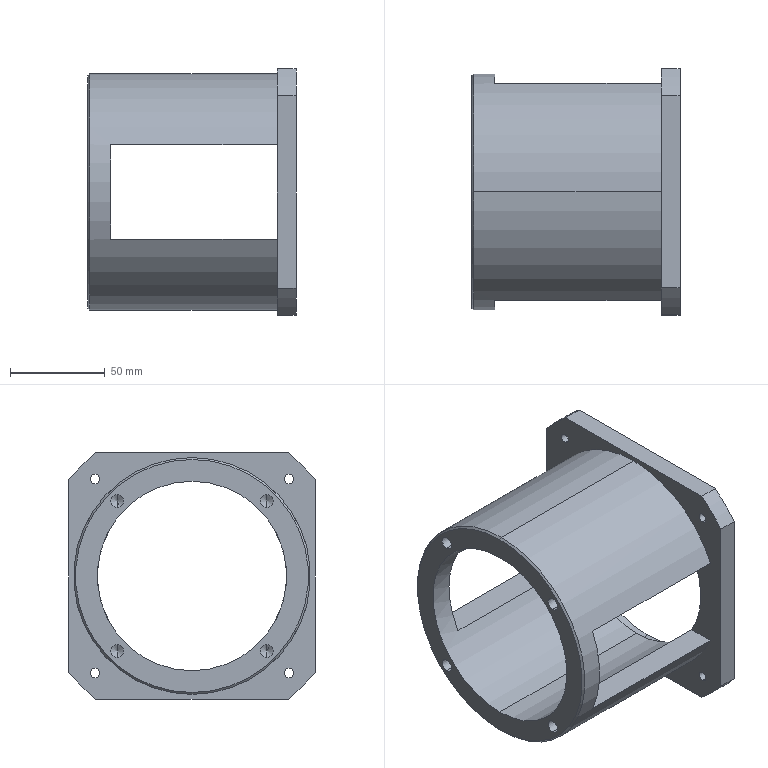Part | SolidWorks | features ICE 5, CirPattern 2, HoleWzd 2, Chamfer 1, Extrusion 1 | 1 solid | 50 faces | box 110 x 130 x 130 mm | volume 397352 mm3 | cylinder 26 | plane 14 | cone 10 | commonest cylinder face diameters 5 x8 6.8 x8 165 x4 100 x2 110 x2 125 x2
STEP:
#1=CARTESIAN_POINT('',(0.,0.,61.5));
#2=VERTEX_POINT('',#1);
#3=CARTESIAN_POINT('',(0.,0.,-61.5));
#4=VERTEX_POINT('',#3);
#5=CARTESIAN_POINT('',(0.,0.,0.));
#6=DIRECTION('',(-1.,0.,0.));
#7=DIRECTION('',(0.,0.,-1.));
#8=AXIS2_PLACEMENT_3D('',#5,#6,#7);
#9=CIRCLE('',#8,61.5);
#10=EDGE_CURVE('',#2,#4,#9,.T.);
#11=ORIENTED_EDGE('',*,*,#10,.F.);
#12=CARTESIAN_POINT('',(1.,0.,62.5));
#13=VERTEX_POINT('',#12);
#14=CARTESIAN_POINT('',(1.,0.,62.5));
#15=DIRECTION('',(0.7071,0.,0.7071));
#16=VECTOR('',#15,1000.);
#17=LINE('',#14,#16);
#18=EDGE_CURVE('',#2,#13,#17,.T.);
#19=ORIENTED_EDGE('',*,*,#18,.T.);
#20=CARTESIAN_POINT('',(1.,0.,-62.5));
#21=VERTEX_POINT('',#20);
#22=CARTESIAN_POINT('',(1.,0.,0.));
#23=DIRECTION('',(1.,0.,0.));
#24=DIRECTION('',(0.,0.,-1.));
#25=AXIS2_PLACEMENT_3D('',#22,#23,#24);
#26=CIRCLE('',#25,62.5);
#27=EDGE_CURVE('',#21,#13,#26,.T.);
#28=ORIENTED_EDGE('',*,*,#27,.F.);
#29=CARTESIAN_POINT('',(1.,0.,-62.5));
#30=DIRECTION('',(0.7071,0.,-0.7071));
#31=VECTOR('',#30,1000.);
#32=LINE('',#29,#31);
#33=EDGE_CURVE('',#4,#21,#32,.T.);
#34=ORIENTED_EDGE('',*,*,#33,.F.);
#35=EDGE_LOOP('',(#11,#19,#28,#34));
#36=FACE_OUTER_BOUND('',#35,.T.);
#37=CARTESIAN_POINT('',(1.,0.,0.));
#38=DIRECTION('',(1.,0.,0.));
#39=DIRECTION('',(0.,0.,-1.));
#40=AXIS2_PLACEMENT_3D('',#37,#38,#39);
#41=CONICAL_SURFACE('',#40,62.5,0.7854);
#42=ADVANCED_FACE('',(#36),#41,.T.);
#43=CARTESIAN_POINT('',(19.75,-39.598,-42.998));
#44=VERTEX_POINT('',#43);
#45=CARTESIAN_POINT('',(19.75,-39.598,-36.198));
#46=VERTEX_POINT('',#45);
#47=CARTESIAN_POINT('',(19.75,-39.598,-39.598));
#48=DIRECTION('',(-1.,0.,0.));
#49=DIRECTION('',(0.,0.,1.));
#50=AXIS2_PLACEMENT_3D('',#47,#48,#49);
#51=CIRCLE('',#50,3.4);
#52=EDGE_CURVE('',#44,#46,#51,.T.);
#53=ORIENTED_EDGE('',*,*,#52,.F.);
#54=CARTESIAN_POINT('',(0.,-39.598,-42.998));
#55=VERTEX_POINT('',#54);
#56=CARTESIAN_POINT('',(0.,-39.598,-42.998));
#57=DIRECTION('',(-1.,0.,0.));
#58=VECTOR('',#57,1000.);
#59=LINE('',#56,#58);
#60=EDGE_CURVE('',#44,#55,#59,.T.);
#61=ORIENTED_EDGE('',*,*,#60,.T.);
#62=CARTESIAN_POINT('',(0.,-39.598,-36.198));
#63=VERTEX_POINT('',#62);
#64=CARTESIAN_POINT('',(0.,-39.598,-39.598));
#65=DIRECTION('',(-1.,0.,0.));
#66=DIRECTION('',(0.,0.,1.));
#67=AXIS2_PLACEMENT_3D('',#64,#65,#66);
#68=CIRCLE('',#67,3.4);
#69=EDGE_CURVE('',#55,#63,#68,.T.);
#70=ORIENTED_EDGE('',*,*,#69,.T.);
#71=CARTESIAN_POINT('',(0.,-39.598,-36.198));
#72=DIRECTION('',(-1.,0.,0.));
#73=VECTOR('',#72,1000.);
#74=LINE('',#71,#73);
#75=EDGE_CURVE('',#46,#63,#74,.T.);
#76=ORIENTED_EDGE('',*,*,#75,.F.);
#77=EDGE_LOOP('',(#53,#61,#70,#76));
#78=FACE_OUTER_BOUND('',#77,.T.);
#79=CARTESIAN_POINT('',(0.,-39.598,-39.598));
#80=DIRECTION('',(-1.,0.,0.));
#81=DIRECTION('',(0.,0.,1.));
#82=AXIS2_PLACEMENT_3D('',#79,#80,#81);
#83=CYLINDRICAL_SURFACE('',#82,3.4);
#84=ADVANCED_FACE('',(#78),#83,.F.);
#85=CARTESIAN_POINT('',(21.793,-39.598,-39.598));
#86=VERTEX_POINT('',#85);
#87=CARTESIAN_POINT('',(19.75,-39.598,-36.198));
#88=DIRECTION('',(-0.515,0.,0.8572));
#89=VECTOR('',#88,1000.);
#90=LINE('',#87,#89);
#91=EDGE_CURVE('',#86,#46,#90,.T.);
#92=ORIENTED_EDGE('',*,*,#91,.F.);
#93=CARTESIAN_POINT('',(19.75,-39.598,-42.998));
#94=DIRECTION('',(-0.515,0.,-0.8572));
#95=VECTOR('',#94,1000.);
#96=LINE('',#93,#95);
#97=EDGE_CURVE('',#86,#44,#96,.T.);
#98=ORIENTED_EDGE('',*,*,#97,.T.);
#99=ORIENTED_EDGE('',*,*,#52,.T.);
#100=EDGE_LOOP('',(#92,#98,#99));
#101=FACE_OUTER_BOUND('',#100,.T.);
#102=CARTESIAN_POINT('',(19.75,-39.598,-39.598));
#103=DIRECTION('',(-1.,0.,0.));
#104=DIRECTION('',(0.,0.,1.));
#105=AXIS2_PLACEMENT_3D('',#102,#103,#104);
#106=CONICAL_SURFACE('',#105,3.4,1.03);
#107=ADVANCED_FACE('',(#101),#106,.F.);
#108=CARTESIAN_POINT('',(19.75,-39.598,36.198));
#109=VERTEX_POINT('',#108);
#110=CARTESIAN_POINT('',(19.75,-39.598,42.998));
#111=VERTEX_POINT('',#110);
#112=CARTESIAN_POINT('',(19.75,-39.598,39.598));
#113=DIRECTION('',(-1.,0.,0.));
#114=DIRECTION('',(0.,0.,1.));
#115=AXIS2_PLACEMENT_3D('',#112,#113,#114);
#116=CIRCLE('',#115,3.4);
#117=EDGE_CURVE('',#109,#111,#116,.T.);
#118=ORIENTED_EDGE('',*,*,#117,.F.);
#119=CARTESIAN_POINT('',(0.,-39.598,36.198));
#120=VERTEX_POINT('',#119);
#121=CARTESIAN_POINT('',(0.,-39.598,36.198));
#122=DIRECTION('',(-1.,0.,0.));
#123=VECTOR('',#122,1000.);
#124=LINE('',#121,#123);
#125=EDGE_CURVE('',#109,#120,#124,.T.);
#126=ORIENTED_EDGE('',*,*,#125,.T.);
#127=CARTESIAN_POINT('',(0.,-39.598,42.998));
#128=VERTEX_POINT('',#127);
#129=CARTESIAN_POINT('',(0.,-39.598,39.598));
#130=DIRECTION('',(-1.,0.,0.));
#131=DIRECTION('',(0.,0.,1.));
#132=AXIS2_PLACEMENT_3D('',#129,#130,#131);
#133=CIRCLE('',#132,3.4);
#134=EDGE_CURVE('',#120,#128,#133,.T.);
#135=ORIENTED_EDGE('',*,*,#134,.T.);
#136=CARTESIAN_POINT('',(0.,-39.598,42.998));
#137=DIRECTION('',(-1.,0.,0.));
#138=VECTOR('',#137,1000.);
#139=LINE('',#136,#138);
#140=EDGE_CURVE('',#111,#128,#139,.T.);
#141=ORIENTED_EDGE('',*,*,#140,.F.);
#142=EDGE_LOOP('',(#118,#126,#135,#141));
#143=FACE_OUTER_BOUND('',#142,.T.);
#144=CARTESIAN_POINT('',(0.,-39.598,39.598));
#145=DIRECTION('',(-1.,0.,0.));
#146=DIRECTION('',(0.,0.,1.));
#147=AXIS2_PLACEMENT_3D('',#144,#145,#146);
#148=CYLINDRICAL_SURFACE('',#147,3.4);
#149=ADVANCED_FACE('',(#143),#148,.F.);
#150=CARTESIAN_POINT('',(21.793,-39.598,39.598));
#151=VERTEX_POINT('',#150);
#152=CARTESIAN_POINT('',(19.75,-39.598,42.998));
#153=DIRECTION('',(-0.515,0.,0.8572));
#154=VECTOR('',#153,1000.);
#155=LINE('',#152,#154);
#156=EDGE_CURVE('',#151,#111,#155,.T.);
#157=ORIENTED_EDGE('',*,*,#156,.F.);
#158=CARTESIAN_POINT('',(19.75,-39.598,36.198));
#159=DIRECTION('',(-0.515,0.,-0.8572));
#160=VECTOR('',#159,1000.);
#161=LINE('',#158,#160);
#162=EDGE_CURVE('',#151,#109,#161,.T.);
#163=ORIENTED_EDGE('',*,*,#162,.T.);
#164=ORIENTED_EDGE('',*,*,#117,.T.);
#165=EDGE_LOOP('',(#157,#163,#164));
#166=FACE_OUTER_BOUND('',#165,.T.);
#167=CARTESIAN_POINT('',(19.75,-39.598,39.598));
#168=DIRECTION('',(-1.,0.,0.));
#169=DIRECTION('',(0.,0.,1.));
#170=AXIS2_PLACEMENT_3D('',#167,#168,#169);
#171=CONICAL_SURFACE('',#170,3.4,1.03);
#172=ADVANCED_FACE('',(#166),#171,.F.);
#173=CARTESIAN_POINT('',(19.75,39.598,36.198));
#174=VERTEX_POINT('',#173);
#175=CARTESIAN_POINT('',(19.75,39.598,42.998));
#176=VERTEX_POINT('',#175);
#177=CARTESIAN_POINT('',(19.75,39.598,39.598));
#178=DIRECTION('',(-1.,0.,0.));
#179=DIRECTION('',(0.,0.,1.));
#180=AXIS2_PLACEMENT_3D('',#177,#178,#179);
#181=CIRCLE('',#180,3.4);
#182=EDGE_CURVE('',#174,#176,#181,.T.);
#183=ORIENTED_EDGE('',*,*,#182,.F.);
#184=CARTESIAN_POINT('',(0.,39.598,36.198));
#185=VERTEX_POINT('',#184);
#186=CARTESIAN_POINT('',(0.,39.598,36.198));
#187=DIRECTION('',(-1.,0.,0.));
#188=VECTOR('',#187,1000.);
#189=LINE('',#186,#188);
#190=EDGE_CURVE('',#174,#185,#189,.T.);
#191=ORIENTED_EDGE('',*,*,#190,.T.);
#192=CARTESIAN_POINT('',(0.,39.598,42.998));
#193=VERTEX_POINT('',#192);
#194=CARTESIAN_POINT('',(0.,39.598,39.598));
#195=DIRECTION('',(-1.,0.,0.));
#196=DIRECTION('',(0.,0.,1.));
#197=AXIS2_PLACEMENT_3D('',#194,#195,#196);
#198=CIRCLE('',#197,3.4);
#199=EDGE_CURVE('',#185,#193,#198,.T.);
#200=ORIENTED_EDGE('',*,*,#199,.T.);
#201=CARTESIAN_POINT('',(0.,39.598,42.998));
#202=DIRECTION('',(-1.,0.,0.));
#203=VECTOR('',#202,1000.);
#204=LINE('',#201,#203);
#205=EDGE_CURVE('',#176,#193,#204,.T.);
#206=ORIENTED_EDGE('',*,*,#205,.F.);
#207=EDGE_LOOP('',(#183,#191,#200,#206));
#208=FACE_OUTER_BOUND('',#207,.T.);
#209=CARTESIAN_POINT('',(0.,39.598,39.598));
#210=DIRECTION('',(-1.,0.,0.));
#211=DIRECTION('',(0.,0.,1.));
#212=AXIS2_PLACEMENT_3D('',#209,#210,#211);
#213=CYLINDRICAL_SURFACE('',#212,3.4);
#214=ADVANCED_FACE('',(#208),#213,.F.);
#215=CARTESIAN_POINT('',(21.793,39.598,39.598));
#216=VERTEX_POINT('',#215);
#217=CARTESIAN_POINT('',(19.75,39.598,42.998));
#218=DIRECTION('',(-0.515,0.,0.8572));
#219=VECTOR('',#218,1000.);
#220=LINE('',#217,#219);
#221=EDGE_CURVE('',#216,#176,#220,.T.);
#222=ORIENTED_EDGE('',*,*,#221,.F.);
#223=CARTESIAN_POINT('',(19.75,39.598,36.198));
#224=DIRECTION('',(-0.515,0.,-0.8572));
#225=VECTOR('',#224,1000.);
#226=LINE('',#223,#225);
#227=EDGE_CURVE('',#216,#174,#226,.T.);
#228=ORIENTED_EDGE('',*,*,#227,.T.);
#229=ORIENTED_EDGE('',*,*,#182,.T.);
#230=EDGE_LOOP('',(#222,#228,#229));
#231=FACE_OUTER_BOUND('',#230,.T.);
#232=CARTESIAN_POINT('',(19.75,39.598,39.598));
#233=DIRECTION('',(-1.,0.,0.));
#234=DIRECTION('',(0.,0.,1.));
#235=AXIS2_PLACEMENT_3D('',#232,#233,#234);
#236=CONICAL_SURFACE('',#235,3.4,1.03);
#237=ADVANCED_FACE('',(#231),#236,.F.);
#238=CARTESIAN_POINT('',(19.75,39.598,-42.998));
#239=VERTEX_POINT('',#238);
#240=CARTESIAN_POINT('',(19.75,39.598,-36.198));
#241=VERTEX_POINT('',#240);
#242=CARTESIAN_POINT('',(19.75,39.598,-39.598));
#243=DIRECTION('',(-1.,0.,0.));
#244=DIRECTION('',(0.,0.,1.));
#245=AXIS2_PLACEMENT_3D('',#242,#243,#244);
#246=CIRCLE('',#245,3.4);
#247=EDGE_CURVE('',#239,#241,#246,.T.);
#248=ORIENTED_EDGE('',*,*,#247,.F.);
#249=CARTESIAN_POINT('',(0.,39.598,-42.998));
#250=VERTEX_POINT('',#249);
#251=CARTESIAN_POINT('',(0.,39.598,-42.998));
#252=DIRECTION('',(-1.,0.,0.));
#253=VECTOR('',#252,1000.);
#254=LINE('',#251,#253);
#255=EDGE_CURVE('',#239,#250,#254,.T.);
#256=ORIENTED_EDGE('',*,*,#255,.T.);
#257=CARTESIAN_POINT('',(0.,39.598,-36.198));
#258=VERTEX_POINT('',#257);
#259=CARTESIAN_POINT('',(0.,39.598,-39.598));
#260=DIRECTION('',(-1.,0.,0.));
#261=DIRECTION('',(0.,0.,1.));
#262=AXIS2_PLACEMENT_3D('',#259,#260,#261);
#263=CIRCLE('',#262,3.4);
#264=EDGE_CURVE('',#250,#258,#263,.T.);
#265=ORIENTED_EDGE('',*,*,#264,.T.);
#266=CARTESIAN_POINT('',(0.,39.598,-36.198));
#267=DIRECTION('',(-1.,0.,0.));
#268=VECTOR('',#267,1000.);
#269=LINE('',#266,#268);
#270=EDGE_CURVE('',#241,#258,#269,.T.);
#271=ORIENTED_EDGE('',*,*,#270,.F.);
#272=EDGE_LOOP('',(#248,#256,#265,#271));
#273=FACE_OUTER_BOUND('',#272,.T.);
#274=CARTESIAN_POINT('',(0.,39.598,-39.598));
#275=DIRECTION('',(-1.,0.,0.));
#276=DIRECTION('',(0.,0.,1.));
#277=AXIS2_PLACEMENT_3D('',#274,#275,#276);
#278=CYLINDRICAL_SURFACE('',#277,3.4);
#279=ADVANCED_FACE('',(#273),#278,.F.);
#280=CARTESIAN_POINT('',(21.793,39.598,-39.598));
#281=VERTEX_POINT('',#280);
#282=CARTESIAN_POINT('',(19.75,39.598,-36.198));
#283=DIRECTION('',(-0.515,0.,0.8572));
#284=VECTOR('',#283,1000.);
#285=LINE('',#282,#284);
#286=EDGE_CURVE('',#281,#241,#285,.T.);
#287=ORIENTED_EDGE('',*,*,#286,.F.);
#288=CARTESIAN_POINT('',(19.75,39.598,-42.998));
#289=DIRECTION('',(-0.515,0.,-0.8572));
#290=VECTOR('',#289,1000.);
#291=LINE('',#288,#290);
#292=EDGE_CURVE('',#281,#239,#291,.T.);
#293=ORIENTED_EDGE('',*,*,#292,.T.);
#294=ORIENTED_EDGE('',*,*,#247,.T.);
#295=EDGE_LOOP('',(#287,#293,#294));
#296=FACE_OUTER_BOUND('',#295,.T.);
#297=CARTESIAN_POINT('',(19.75,39.598,-39.598));
#298=DIRECTION('',(-1.,0.,0.));
#299=DIRECTION('',(0.,0.,1.));
#300=AXIS2_PLACEMENT_3D('',#297,#298,#299);
#301=CONICAL_SURFACE('',#300,3.4,1.03);
#302=ADVANCED_FACE('',(#296),#301,.F.);
#303=CARTESIAN_POINT('',(100.,-43.301,25.));
#304=VERTEX_POINT('',#303);
#305=CARTESIAN_POINT('',(12.,-43.301,25.));
#306=VERTEX_POINT('',#305);
#307=CARTESIAN_POINT('',(0.,-43.301,25.));
#308=DIRECTION('',(-1.,0.,0.));
#309=VECTOR('',#308,1000.);
#310=LINE('',#307,#309);
#311=EDGE_CURVE('',#304,#306,#310,.T.);
#312=ORIENTED_EDGE('',*,*,#311,.T.);
#313=CARTESIAN_POINT('',(12.,-43.301,-25.));
#314=VERTEX_POINT('',#313);
#315=CARTESIAN_POINT('',(12.,0.,0.));
#316=DIRECTION('',(1.,0.,0.));
#317=DIRECTION('',(0.,0.,1.));
#318=AXIS2_PLACEMENT_3D('',#315,#316,#317);
#319=CIRCLE('',#318,50.);
#320=EDGE_CURVE('',#306,#314,#319,.T.);
#321=ORIENTED_EDGE('',*,*,#320,.T.);
#322=CARTESIAN_POINT('',(100.,-43.301,-25.));
#323=VERTEX_POINT('',#322);
#324=CARTESIAN_POINT('',(0.,-43.301,-25.));
#325=DIRECTION('',(1.,0.,0.));
#326=VECTOR('',#325,1000.);
#327=LINE('',#324,#326);
#328=EDGE_CURVE('',#314,#323,#327,.T.);
#329=ORIENTED_EDGE('',*,*,#328,.T.);
#330=CARTESIAN_POINT('',(100.,0.,0.));
#331=DIRECTION('',(-1.,0.,0.));
#332=DIRECTION('',(0.,0.,-1.));
#333=AXIS2_PLACEMENT_3D('',#330,#331,#332);
#334=CIRCLE('',#333,50.);
#335=EDGE_CURVE('',#323,#304,#334,.T.);
#336=ORIENTED_EDGE('',*,*,#335,.T.);
#337=EDGE_LOOP('',(#312,#321,#329,#336));
#338=FACE_BOUND('',#337,.T.);
#339=CARTESIAN_POINT('',(0.,0.,50.));
#340=VERTEX_POINT('',#339);
#341=CARTESIAN_POINT('',(0.,0.,-50.));
#342=VERTEX_POINT('',#341);
#343=CARTESIAN_POINT('',(0.,0.,0.));
#344=DIRECTION('',(1.,0.,0.));
#345=DIRECTION('',(0.,0.,-1.));
#346=AXIS2_PLACEMENT_3D('',#343,#344,#345);
#347=CIRCLE('',#346,50.);
#348=EDGE_CURVE('',#340,#342,#347,.T.);
#349=ORIENTED_EDGE('',*,*,#348,.F.);
#350=CARTESIAN_POINT('',(102.,0.,50.));
#351=VERTEX_POINT('',#350);
#352=CARTESIAN_POINT('',(0.,0.,50.));
#353=DIRECTION('',(1.,0.,0.));
#354=VECTOR('',#353,1000.);
#355=LINE('',#352,#354);
#356=EDGE_CURVE('',#340,#351,#355,.T.);
#357=ORIENTED_EDGE('',*,*,#356,.T.);
#358=CARTESIAN_POINT('',(102.,0.,-50.));
#359=VERTEX_POINT('',#358);
#360=CARTESIAN_POINT('',(102.,0.,0.));
#361=DIRECTION('',(1.,0.,0.));
#362=DIRECTION('',(0.,0.,-1.));
#363=AXIS2_PLACEMENT_3D('',#360,#361,#362);
#364=CIRCLE('',#363,50.);
#365=EDGE_CURVE('',#351,#359,#364,.T.);
#366=ORIENTED_EDGE('',*,*,#365,.T.);
#367=CARTESIAN_POINT('',(0.,0.,-50.));
#368=DIRECTION('',(1.,0.,0.));
#369=VECTOR('',#368,1000.);
#370=LINE('',#367,#369);
#371=EDGE_CURVE('',#342,#359,#370,.T.);
#372=ORIENTED_EDGE('',*,*,#371,.F.);
#373=EDGE_LOOP('',(#349,#357,#366,#372));
#374=FACE_OUTER_BOUND('',#373,.T.);
#375=CARTESIAN_POINT('',(0.,0.,0.));
#376=DIRECTION('',(1.,0.,0.));
#377=DIRECTION('',(0.,0.,-1.));
#378=AXIS2_PLACEMENT_3D('',#375,#376,#377);
#379=CYLINDRICAL_SURFACE('',#378,50.);
#380=ADVANCED_FACE('',(#338,#374),#379,.F.);
#381=CARTESIAN_POINT('',(100.,-51.265,53.765));
#382=VERTEX_POINT('',#381);
#383=CARTESIAN_POINT('',(100.,-51.265,48.765));
#384=VERTEX_POINT('',#383);
#385=CARTESIAN_POINT('',(100.,-51.265,51.265));
#386=DIRECTION('',(1.,0.,0.));
#387=DIRECTION('',(0.,0.,-1.));
#388=AXIS2_PLACEMENT_3D('',#385,#386,#387);
#389=CIRCLE('',#388,2.5);
#390=EDGE_CURVE('',#382,#384,#389,.T.);
#391=ORIENTED_EDGE('',*,*,#390,.F.);
#392=CARTESIAN_POINT('',(110.,-51.265,53.765));
#393=VERTEX_POINT('',#392);
#394=CARTESIAN_POINT('',(110.,-51.265,53.765));
#395=DIRECTION('',(1.,0.,0.));
#396=VECTOR('',#395,1000.);
#397=LINE('',#394,#396);
#398=EDGE_CURVE('',#382,#393,#397,.T.);
#399=ORIENTED_EDGE('',*,*,#398,.T.);
#400=CARTESIAN_POINT('',(110.,-51.265,48.765));
#401=VERTEX_POINT('',#400);
#402=CARTESIAN_POINT('',(110.,-51.265,51.265));
#403=DIRECTION('',(1.,0.,0.));
#404=DIRECTION('',(0.,0.,-1.));
#405=AXIS2_PLACEMENT_3D('',#402,#403,#404);
#406=CIRCLE('',#405,2.5);
#407=EDGE_CURVE('',#393,#401,#406,.T.);
#408=ORIENTED_EDGE('',*,*,#407,.T.);
#409=CARTESIAN_POINT('',(110.,-51.265,48.765));
#410=DIRECTION('',(1.,0.,0.));
#411=VECTOR('',#410,1000.);
#412=LINE('',#409,#411);
#413=EDGE_CURVE('',#384,#401,#412,.T.);
#414=ORIENTED_EDGE('',*,*,#413,.F.);
#415=EDGE_LOOP('',(#391,#399,#408,#414));
#416=FACE_OUTER_BOUND('',#415,.T.);
#417=CARTESIAN_POINT('',(110.,-51.265,51.265));
#418=DIRECTION('',(1.,0.,0.));
#419=DIRECTION('',(0.,0.,-1.));
#420=AXIS2_PLACEMENT_3D('',#417,#418,#419);
#421=CYLINDRICAL_SURFACE('',#420,2.5);
#422=ADVANCED_FACE('',(#416),#421,.F.);
#423=CARTESIAN_POINT('',(100.,-51.265,-48.765));
#424=VERTEX_POINT('',#423);
#425=CARTESIAN_POINT('',(100.,-51.265,-53.765));
#426=VERTEX_POINT('',#425);
#427=CARTESIAN_POINT('',(100.,-51.265,-51.265));
#428=DIRECTION('',(1.,0.,0.));
#429=DIRECTION('',(0.,0.,-1.));
#430=AXIS2_PLACEMENT_3D('',#427,#428,#429);
#431=CIRCLE('',#430,2.5);
#432=EDGE_CURVE('',#424,#426,#431,.T.);
#433=ORIENTED_EDGE('',*,*,#432,.F.);
#434=CARTESIAN_POINT('',(110.,-51.265,-48.765));
#435=VERTEX_POINT('',#434);
#436=CARTESIAN_POINT('',(110.,-51.265,-48.765));
#437=DIRECTION('',(1.,0.,0.));
#438=VECTOR('',#437,1000.);
#439=LINE('',#436,#438);
#440=EDGE_CURVE('',#424,#435,#439,.T.);
#441=ORIENTED_EDGE('',*,*,#440,.T.);
#442=CARTESIAN_POINT('',(110.,-51.265,-53.765));
#443=VERTEX_POINT('',#442);
#444=CARTESIAN_POINT('',(110.,-51.265,-51.265));
#445=DIRECTION('',(1.,0.,0.));
#446=DIRECTION('',(0.,0.,-1.));
#447=AXIS2_PLACEMENT_3D('',#444,#445,#446);
#448=CIRCLE('',#447,2.5);
#449=EDGE_CURVE('',#435,#443,#448,.T.);
#450=ORIENTED_EDGE('',*,*,#449,.T.);
#451=CARTESIAN_POINT('',(110.,-51.265,-53.765));
#452=DIRECTION('',(1.,0.,0.));
#453=VECTOR('',#452,1000.);
#454=LINE('',#451,#453);
#455=EDGE_CURVE('',#426,#443,#454,.T.);
#456=ORIENTED_EDGE('',*,*,#455,.F.);
#457=EDGE_LOOP('',(#433,#441,#450,#456));
#458=FACE_OUTER_BOUND('',#457,.T.);
#459=CARTESIAN_POINT('',(110.,-51.265,-51.265));
#460=DIRECTION('',(1.,0.,0.));
#461=DIRECTION('',(0.,0.,-1.));
#462=AXIS2_PLACEMENT_3D('',#459,#460,#461);
#463=CYLINDRICAL_SURFACE('',#462,2.5);
#464=ADVANCED_FACE('',(#458),#463,.F.);
#465=CARTESIAN_POINT('',(100.,51.265,-48.765));
#466=VERTEX_POINT('',#465);
#467=CARTESIAN_POINT('',(100.,51.265,-53.765));
#468=VERTEX_POINT('',#467);
#469=CARTESIAN_POINT('',(100.,51.265,-51.265));
#470=DIRECTION('',(1.,0.,0.));
#471=DIRECTION('',(0.,0.,-1.));
#472=AXIS2_PLACEMENT_3D('',#469,#470,#471);
#473=CIRCLE('',#472,2.5);
#474=EDGE_CURVE('',#466,#468,#473,.T.);
#475=ORIENTED_EDGE('',*,*,#474,.F.);
#476=CARTESIAN_POINT('',(110.,51.265,-48.765));
#477=VERTEX_POINT('',#476);
#478=CARTESIAN_POINT('',(110.,51.265,-48.765));
#479=DIRECTION('',(1.,0.,0.));
#480=VECTOR('',#479,1000.);
#481=LINE('',#478,#480);
#482=EDGE_CURVE('',#466,#477,#481,.T.);
#483=ORIENTED_EDGE('',*,*,#482,.T.);
#484=CARTESIAN_POINT('',(110.,51.265,-53.765));
#485=VERTEX_POINT('',#484);
#486=CARTESIAN_POINT('',(110.,51.265,-51.265));
#487=DIRECTION('',(1.,0.,0.));
#488=DIRECTION('',(0.,0.,-1.));
#489=AXIS2_PLACEMENT_3D('',#486,#487,#488);
#490=CIRCLE('',#489,2.5);
#491=EDGE_CURVE('',#477,#485,#490,.T.);
#492=ORIENTED_EDGE('',*,*,#491,.T.);
#493=CARTESIAN_POINT('',(110.,51.265,-53.765));
#494=DIRECTION('',(1.,0.,0.));
#495=VECTOR('',#494,1000.);
#496=LINE('',#493,#495);
#497=EDGE_CURVE('',#468,#485,#496,.T.);
#498=ORIENTED_EDGE('',*,*,#497,.F.);
#499=EDGE_LOOP('',(#475,#483,#492,#498));
#500=FACE_OUTER_BOUND('',#499,.T.);
#501=CARTESIAN_POINT('',(110.,51.265,-51.265));
#502=DIRECTION('',(1.,0.,0.));
#503=DIRECTION('',(0.,0.,-1.));
#504=AXIS2_PLACEMENT_3D('',#501,#502,#503);
#505=CYLINDRICAL_SURFACE('',#504,2.5);
#506=ADVANCED_FACE('',(#500),#505,.F.);
#507=CARTESIAN_POINT('',(100.,51.265,53.765));
#508=VERTEX_POINT('',#507);
#509=CARTESIAN_POINT('',(100.,51.265,48.765));
#510=VERTEX_POINT('',#509);
#511=CARTESIAN_POINT('',(100.,51.265,51.265));
#512=DIRECTION('',(1.,0.,0.));
#513=DIRECTION('',(0.,0.,-1.));
#514=AXIS2_PLACEMENT_3D('',#511,#512,#513);
#515=CIRCLE('',#514,2.5);
#516=EDGE_CURVE('',#508,#510,#515,.T.);
#517=ORIENTED_EDGE('',*,*,#516,.F.);
#518=CARTESIAN_POINT('',(110.,51.265,53.765));
#519=VERTEX_POINT('',#518);
#520=CARTESIAN_POINT('',(110.,51.265,53.765));
#521=DIRECTION('',(1.,0.,0.));
#522=VECTOR('',#521,1000.);
#523=LINE('',#520,#522);
#524=EDGE_CURVE('',#508,#519,#523,.T.);
#525=ORIENTED_EDGE('',*,*,#524,.T.);
#526=CARTESIAN_POINT('',(110.,51.265,48.765));
#527=VERTEX_POINT('',#526);
#528=CARTESIAN_POINT('',(110.,51.265,51.265));
#529=DIRECTION('',(1.,0.,0.));
#530=DIRECTION('',(0.,0.,-1.));
#531=AXIS2_PLACEMENT_3D('',#528,#529,#530);
#532=CIRCLE('',#531,2.5);
#533=EDGE_CURVE('',#519,#527,#532,.T.);
#534=ORIENTED_EDGE('',*,*,#533,.T.);
#535=CARTESIAN_POINT('',(110.,51.265,48.765));
#536=DIRECTION('',(1.,0.,0.));
#537=VECTOR('',#536,1000.);
#538=LINE('',#535,#537);
#539=EDGE_CURVE('',#510,#527,#538,.T.);
#540=ORIENTED_EDGE('',*,*,#539,.F.);
#541=EDGE_LOOP('',(#517,#525,#534,#540));
#542=FACE_OUTER_BOUND('',#541,.T.);
#543=CARTESIAN_POINT('',(110.,51.265,51.265));
#544=DIRECTION('',(1.,0.,0.));
#545=DIRECTION('',(0.,0.,-1.));
#546=AXIS2_PLACEMENT_3D('',#543,#544,#545);
#547=CYLINDRICAL_SURFACE('',#546,2.5);
#548=ADVANCED_FACE('',(#542),#547,.F.);
#549=CARTESIAN_POINT('',(102.,0.,55.));
#550=VERTEX_POINT('',#549);
#551=CARTESIAN_POINT('',(102.,0.,-55.));
#552=VERTEX_POINT('',#551);
#553=CARTESIAN_POINT('',(102.,0.,0.));
#554=DIRECTION('',(1.,0.,0.));
#555=DIRECTION('',(0.,0.,-1.));
#556=AXIS2_PLACEMENT_3D('',#553,#554,#555);
#557=CIRCLE('',#556,55.);
#558=EDGE_CURVE('',#550,#552,#557,.T.);
#559=ORIENTED_EDGE('',*,*,#558,.F.);
#560=CARTESIAN_POINT('',(110.,0.,55.));
#561=VERTEX_POINT('',#560);
#562=CARTESIAN_POINT('',(102.,0.,55.));
#563=DIRECTION('',(1.,0.,0.));
#564=VECTOR('',#563,1000.);
#565=LINE('',#562,#564);
#566=EDGE_CURVE('',#550,#561,#565,.T.);
#567=ORIENTED_EDGE('',*,*,#566,.T.);
#568=CARTESIAN_POINT('',(110.,0.,-55.));
#569=VERTEX_POINT('',#568);
#570=CARTESIAN_POINT('',(110.,0.,0.));
#571=DIRECTION('',(1.,0.,0.));
#572=DIRECTION('',(0.,0.,-1.));
#573=AXIS2_PLACEMENT_3D('',#570,#571,#572);
#574=CIRCLE('',#573,55.);
#575=EDGE_CURVE('',#561,#569,#574,.T.);
#576=ORIENTED_EDGE('',*,*,#575,.T.);
#577=CARTESIAN_POINT('',(102.,0.,-55.));
#578=DIRECTION('',(1.,0.,0.));
#579=VECTOR('',#578,1000.);
#580=LINE('',#577,#579);
#581=EDGE_CURVE('',#552,#569,#580,.T.);
#582=ORIENTED_EDGE('',*,*,#581,.F.);
#583=EDGE_LOOP('',(#559,#567,#576,#582));
#584=FACE_OUTER_BOUND('',#583,.T.);
#585=CARTESIAN_POINT('',(102.,0.,0.));
#586=DIRECTION('',(1.,0.,0.));
#587=DIRECTION('',(0.,0.,-1.));
#588=AXIS2_PLACEMENT_3D('',#585,#586,#587);
#589=CYLINDRICAL_SURFACE('',#588,55.);
#590=ADVANCED_FACE('',(#584),#589,.F.);
#591=CARTESIAN_POINT('',(100.,0.,-62.5));
#592=VERTEX_POINT('',#591);
#593=CARTESIAN_POINT('',(100.,57.282,-25.));
#594=VERTEX_POINT('',#593);
#595=CARTESIAN_POINT('',(100.,0.,0.));
#596=DIRECTION('',(1.,0.,0.));
#597=DIRECTION('',(0.,0.,-1.));
#598=AXIS2_PLACEMENT_3D('',#595,#596,#597);
#599=CIRCLE('',#598,62.5);
#600=EDGE_CURVE('',#592,#594,#599,.T.);
#601=ORIENTED_EDGE('',*,*,#600,.F.);
#602=CARTESIAN_POINT('',(100.,0.,-62.5));
#603=DIRECTION('',(-1.,0.,0.));
#604=VECTOR('',#603,1000.);
#605=LINE('',#602,#604);
#606=EDGE_CURVE('',#592,#21,#605,.T.);
#607=ORIENTED_EDGE('',*,*,#606,.T.);
#608=ORIENTED_EDGE('',*,*,#27,.T.);
#609=CARTESIAN_POINT('',(100.,0.,62.5));
#610=VERTEX_POINT('',#609);
#611=CARTESIAN_POINT('',(100.,0.,62.5));
#612=DIRECTION('',(-1.,0.,0.));
#613=VECTOR('',#612,1000.);
#614=LINE('',#611,#613);
#615=EDGE_CURVE('',#610,#13,#614,.T.);
#616=ORIENTED_EDGE('',*,*,#615,.F.);
#617=CARTESIAN_POINT('',(100.,57.282,25.));
#618=VERTEX_POINT('',#617);
#619=CARTESIAN_POINT('',(100.,0.,0.));
#620=DIRECTION('',(1.,0.,0.));
#621=DIRECTION('',(0.,0.,-1.));
#622=AXIS2_PLACEMENT_3D('',#619,#620,#621);
#623=CIRCLE('',#622,62.5);
#624=EDGE_CURVE('',#618,#610,#623,.T.);
#625=ORIENTED_EDGE('',*,*,#624,.F.);
#626=CARTESIAN_POINT('',(12.,57.282,25.));
#627=VERTEX_POINT('',#626);
#628=CARTESIAN_POINT('',(100.,57.282,25.));
#629=DIRECTION('',(-1.,0.,0.));
#630=VECTOR('',#629,1000.);
#631=LINE('',#628,#630);
#632=EDGE_CURVE('',#618,#627,#631,.T.);
#633=ORIENTED_EDGE('',*,*,#632,.T.);
#634=CARTESIAN_POINT('',(12.,57.282,-25.));
#635=VERTEX_POINT('',#634);
#636=CARTESIAN_POINT('',(12.,0.,0.));
#637=DIRECTION('',(-1.,0.,0.));
#638=DIRECTION('',(0.,0.,1.));
#639=AXIS2_PLACEMENT_3D('',#636,#637,#638);
#640=CIRCLE('',#639,62.5);
#641=EDGE_CURVE('',#627,#635,#640,.T.);
#642=ORIENTED_EDGE('',*,*,#641,.T.);
#643=CARTESIAN_POINT('',(100.,57.282,-25.));
#644=DIRECTION('',(1.,0.,0.));
#645=VECTOR('',#644,1000.);
#646=LINE('',#643,#645);
#647=EDGE_CURVE('',#635,#594,#646,.T.);
#648=ORIENTED_EDGE('',*,*,#647,.T.);
#649=EDGE_LOOP('',(#601,#607,#608,#616,#625,#633,#642,#648));
#650=FACE_OUTER_BOUND('',#649,.T.);
#651=CARTESIAN_POINT('',(100.,0.,0.));
#652=DIRECTION('',(-1.,0.,0.));
#653=DIRECTION('',(0.,0.,1.));
#654=AXIS2_PLACEMENT_3D('',#651,#652,#653);
#655=CYLINDRICAL_SURFACE('',#654,62.5);
#656=ADVANCED_FACE('',(#650),#655,.T.);
#657=CARTESIAN_POINT('',(110.,50.806,65.));
#658=VERTEX_POINT('',#657);
#659=CARTESIAN_POINT('',(100.,50.806,65.));
#660=VERTEX_POINT('',#659);
#661=CARTESIAN_POINT('',(110.,50.806,65.));
#662=DIRECTION('',(-1.,0.,0.));
#663=VECTOR('',#662,1000.);
#664=LINE('',#661,#663);
#665=EDGE_CURVE('',#658,#660,#664,.T.);
#666=ORIENTED_EDGE('',*,*,#665,.F.);
#667=CARTESIAN_POINT('',(110.,65.,50.806));
#668=VERTEX_POINT('',#667);
#669=CARTESIAN_POINT('',(110.,0.,0.));
#670=DIRECTION('',(1.,0.,0.));
#671=DIRECTION('',(0.,0.,-1.));
#672=AXIS2_PLACEMENT_3D('',#669,#670,#671);
#673=CIRCLE('',#672,82.5);
#674=EDGE_CURVE('',#668,#658,#673,.T.);
#675=ORIENTED_EDGE('',*,*,#674,.F.);
#676=CARTESIAN_POINT('',(100.,65.,50.806));
#677=VERTEX_POINT('',#676);
#678=CARTESIAN_POINT('',(110.,65.,50.806));
#679=DIRECTION('',(1.,0.,0.));
#680=VECTOR('',#679,1000.);
#681=LINE('',#678,#680);
#682=EDGE_CURVE('',#677,#668,#681,.T.);
#683=ORIENTED_EDGE('',*,*,#682,.F.);
#684=CARTESIAN_POINT('',(100.,0.,0.));
#685=DIRECTION('',(1.,0.,0.));
#686=DIRECTION('',(0.,0.,-1.));
#687=AXIS2_PLACEMENT_3D('',#684,#685,#686);
#688=CIRCLE('',#687,82.5);
#689=EDGE_CURVE('',#677,#660,#688,.T.);
#690=ORIENTED_EDGE('',*,*,#689,.T.);
#691=EDGE_LOOP('',(#666,#675,#683,#690));
#692=FACE_OUTER_BOUND('',#691,.T.);
#693=CARTESIAN_POINT('',(110.,0.,0.));
#694=DIRECTION('',(-1.,0.,0.));
#695=DIRECTION('',(0.,0.,1.));
#696=AXIS2_PLACEMENT_3D('',#693,#694,#695);
#697=CYLINDRICAL_SURFACE('',#696,82.5);
#698=ADVANCED_FACE('',(#692),#697,.T.);
#699=CARTESIAN_POINT('',(100.,-50.806,65.));
#700=VERTEX_POINT('',#699);
#701=CARTESIAN_POINT('',(110.,-50.806,65.));
#702=VERTEX_POINT('',#701);
#703=CARTESIAN_POINT('',(110.,-50.806,65.));
#704=DIRECTION('',(1.,0.,0.));
#705=VECTOR('',#704,1000.);
#706=LINE('',#703,#705);
#707=EDGE_CURVE('',#700,#702,#706,.T.);
#708=ORIENTED_EDGE('',*,*,#707,.F.);
#709=CARTESIAN_POINT('',(100.,-65.,50.806));
#710=VERTEX_POINT('',#709);
#711=CARTESIAN_POINT('',(100.,0.,0.));
#712=DIRECTION('',(1.,0.,0.));
#713=DIRECTION('',(0.,0.,-1.));
#714=AXIS2_PLACEMENT_3D('',#711,#712,#713);
#715=CIRCLE('',#714,82.5);
#716=EDGE_CURVE('',#700,#710,#715,.T.);
#717=ORIENTED_EDGE('',*,*,#716,.T.);
#718=CARTESIAN_POINT('',(110.,-65.,50.806));
#719=VERTEX_POINT('',#718);
#720=CARTESIAN_POINT('',(110.,-65.,50.806));
#721=DIRECTION('',(-1.,0.,0.));
#722=VECTOR('',#721,1000.);
#723=LINE('',#720,#722);
#724=EDGE_CURVE('',#719,#710,#723,.T.);
#725=ORIENTED_EDGE('',*,*,#724,.F.);
#726=CARTESIAN_POINT('',(110.,0.,0.));
#727=DIRECTION('',(1.,0.,0.));
#728=DIRECTION('',(0.,0.,-1.));
#729=AXIS2_PLACEMENT_3D('',#726,#727,#728);
#730=CIRCLE('',#729,82.5);
#731=EDGE_CURVE('',#702,#719,#730,.T.);
#732=ORIENTED_EDGE('',*,*,#731,.F.);
#733=EDGE_LOOP('',(#708,#717,#725,#732));
#734=FACE_OUTER_BOUND('',#733,.T.);
#735=CARTESIAN_POINT('',(110.,0.,0.));
#736=DIRECTION('',(-1.,0.,0.));
#737=DIRECTION('',(0.,0.,1.));
#738=AXIS2_PLACEMENT_3D('',#735,#736,#737);
#739=CYLINDRICAL_SURFACE('',#738,82.5);
#740=ADVANCED_FACE('',(#734),#739,.T.);
#741=CARTESIAN_POINT('',(110.,65.,-50.806));
#742=VERTEX_POINT('',#741);
#743=CARTESIAN_POINT('',(100.,65.,-50.806));
#744=VERTEX_POINT('',#743);
#745=CARTESIAN_POINT('',(110.,65.,-50.806));
#746=DIRECTION('',(-1.,0.,0.));
#747=VECTOR('',#746,1000.);
#748=LINE('',#745,#747);
#749=EDGE_CURVE('',#742,#744,#748,.T.);
#750=ORIENTED_EDGE('',*,*,#749,.F.);
#751=CARTESIAN_POINT('',(110.,50.806,-65.));
#752=VERTEX_POINT('',#751);
#753=CARTESIAN_POINT('',(110.,0.,0.));
#754=DIRECTION('',(1.,0.,0.));
#755=DIRECTION('',(0.,0.,-1.));
#756=AXIS2_PLACEMENT_3D('',#753,#754,#755);
#757=CIRCLE('',#756,82.5);
#758=EDGE_CURVE('',#752,#742,#757,.T.);
#759=ORIENTED_EDGE('',*,*,#758,.F.);
#760=CARTESIAN_POINT('',(100.,50.806,-65.));
#761=VERTEX_POINT('',#760);
#762=CARTESIAN_POINT('',(110.,50.806,-65.));
#763=DIRECTION('',(1.,0.,0.));
#764=VECTOR('',#763,1000.);
#765=LINE('',#762,#764);
#766=EDGE_CURVE('',#761,#752,#765,.T.);
#767=ORIENTED_EDGE('',*,*,#766,.F.);
#768=CARTESIAN_POINT('',(100.,0.,0.));
#769=DIRECTION('',(1.,0.,0.));
#770=DIRECTION('',(0.,0.,-1.));
#771=AXIS2_PLACEMENT_3D('',#768,#769,#770);
#772=CIRCLE('',#771,82.5);
#773=EDGE_CURVE('',#761,#744,#772,.T.);
#774=ORIENTED_EDGE('',*,*,#773,.T.);
#775=EDGE_LOOP('',(#750,#759,#767,#774));
#776=FACE_OUTER_BOUND('',#775,.T.);
#777=CARTESIAN_POINT('',(110.,0.,0.));
#778=DIRECTION('',(-1.,0.,0.));
#779=DIRECTION('',(0.,0.,1.));
#780=AXIS2_PLACEMENT_3D('',#777,#778,#779);
#781=CYLINDRICAL_SURFACE('',#780,82.5);
#782=ADVANCED_FACE('',(#776),#781,.T.);
#783=CARTESIAN_POINT('',(110.,-50.806,-65.));
#784=VERTEX_POINT('',#783);
#785=CARTESIAN_POINT('',(100.,-50.806,-65.));
#786=VERTEX_POINT('',#785);
#787=CARTESIAN_POINT('',(110.,-50.806,-65.));
#788=DIRECTION('',(-1.,0.,0.));
#789=VECTOR('',#788,1000.);
#790=LINE('',#787,#789);
#791=EDGE_CURVE('',#784,#786,#790,.T.);
#792=ORIENTED_EDGE('',*,*,#791,.F.);
#793=CARTESIAN_POINT('',(110.,-65.,-50.806));
#794=VERTEX_POINT('',#793);
#795=CARTESIAN_POINT('',(110.,0.,0.));
#796=DIRECTION('',(1.,0.,0.));
#797=DIRECTION('',(0.,0.,-1.));
#798=AXIS2_PLACEMENT_3D('',#795,#796,#797);
#799=CIRCLE('',#798,82.5);
#800=EDGE_CURVE('',#794,#784,#799,.T.);
#801=ORIENTED_EDGE('',*,*,#800,.F.);
#802=CARTESIAN_POINT('',(100.,-65.,-50.806));
#803=VERTEX_POINT('',#802);
#804=CARTESIAN_POINT('',(110.,-65.,-50.806));
#805=DIRECTION('',(1.,0.,0.));
#806=VECTOR('',#805,1000.);
#807=LINE('',#804,#806);
#808=EDGE_CURVE('',#803,#794,#807,.T.);
#809=ORIENTED_EDGE('',*,*,#808,.F.);
#810=CARTESIAN_POINT('',(100.,0.,0.));
#811=DIRECTION('',(1.,0.,0.));
#812=DIRECTION('',(0.,0.,-1.));
#813=AXIS2_PLACEMENT_3D('',#810,#811,#812);
#814=CIRCLE('',#813,82.5);
#815=EDGE_CURVE('',#803,#786,#814,.T.);
#816=ORIENTED_EDGE('',*,*,#815,.T.);
#817=EDGE_LOOP('',(#792,#801,#809,#816));
#818=FACE_OUTER_BOUND('',#817,.T.);
#819=CARTESIAN_POINT('',(110.,0.,0.));
#820=DIRECTION('',(-1.,0.,0.));
#821=DIRECTION('',(0.,0.,1.));
#822=AXIS2_PLACEMENT_3D('',#819,#820,#821);
#823=CYLINDRICAL_SURFACE('',#822,82.5);
#824=ADVANCED_FACE('',(#818),#823,.T.);
#825=CARTESIAN_POINT('',(110.,-51.265,51.265));
#826=DIRECTION('',(1.,0.,0.));
#827=DIRECTION('',(0.,0.,-1.));
#828=AXIS2_PLACEMENT_3D('',#825,#826,#827);
#829=CIRCLE('',#828,2.5);
#830=EDGE_CURVE('',#401,#393,#829,.T.);
#831=ORIENTED_EDGE('',*,*,#830,.F.);
#832=ORIENTED_EDGE('',*,*,#407,.F.);
#833=EDGE_LOOP('',(#831,#832));
#834=FACE_BOUND('',#833,.T.);
#835=CARTESIAN_POINT('',(110.,-51.265,-51.265));
#836=DIRECTION('',(1.,0.,0.));
#837=DIRECTION('',(0.,0.,-1.));
#838=AXIS2_PLACEMENT_3D('',#835,#836,#837);
#839=CIRCLE('',#838,2.5);
#840=EDGE_CURVE('',#443,#435,#839,.T.);
#841=ORIENTED_EDGE('',*,*,#840,.F.);
#842=ORIENTED_EDGE('',*,*,#449,.F.);
#843=EDGE_LOOP('',(#841,#842));
#844=FACE_BOUND('',#843,.T.);
#845=CARTESIAN_POINT('',(110.,51.265,-51.265));
#846=DIRECTION('',(1.,0.,0.));
#847=DIRECTION('',(0.,0.,-1.));
#848=AXIS2_PLACEMENT_3D('',#845,#846,#847);
#849=CIRCLE('',#848,2.5);
#850=EDGE_CURVE('',#485,#477,#849,.T.);
#851=ORIENTED_EDGE('',*,*,#850,.F.);
#852=ORIENTED_EDGE('',*,*,#491,.F.);
#853=EDGE_LOOP('',(#851,#852));
#854=FACE_BOUND('',#853,.T.);
#855=CARTESIAN_POINT('',(110.,51.265,51.265));
#856=DIRECTION('',(1.,0.,0.));
#857=DIRECTION('',(0.,0.,-1.));
#858=AXIS2_PLACEMENT_3D('',#855,#856,#857);
#859=CIRCLE('',#858,2.5);
#860=EDGE_CURVE('',#527,#519,#859,.T.);
#861=ORIENTED_EDGE('',*,*,#860,.F.);
#862=ORIENTED_EDGE('',*,*,#533,.F.);
#863=EDGE_LOOP('',(#861,#862));
#864=FACE_BOUND('',#863,.T.);
#865=CARTESIAN_POINT('',(110.,0.,0.));
#866=DIRECTION('',(1.,0.,0.));
#867=DIRECTION('',(0.,0.,-1.));
#868=AXIS2_PLACEMENT_3D('',#865,#866,#867);
#869=CIRCLE('',#868,55.);
#870=EDGE_CURVE('',#569,#561,#869,.T.);
#871=ORIENTED_EDGE('',*,*,#870,.F.);
#872=ORIENTED_EDGE('',*,*,#575,.F.);
#873=EDGE_LOOP('',(#871,#872));
#874=FACE_BOUND('',#873,.T.);
#875=ORIENTED_EDGE('',*,*,#674,.T.);
#876=CARTESIAN_POINT('',(110.,65.,65.));
#877=DIRECTION('',(0.,-1.,0.));
#878=VECTOR('',#877,1000.);
#879=LINE('',#876,#878);
#880=EDGE_CURVE('',#658,#702,#879,.T.);
#881=ORIENTED_EDGE('',*,*,#880,.T.);
#882=ORIENTED_EDGE('',*,*,#731,.T.);
#883=CARTESIAN_POINT('',(110.,-65.,65.));
#884=DIRECTION('',(0.,0.,-1.));
#885=VECTOR('',#884,1000.);
#886=LINE('',#883,#885);
#887=EDGE_CURVE('',#719,#794,#886,.T.);
#888=ORIENTED_EDGE('',*,*,#887,.T.);
#889=ORIENTED_EDGE('',*,*,#800,.T.);
#890=CARTESIAN_POINT('',(110.,65.,-65.));
#891=DIRECTION('',(0.,1.,0.));
#892=VECTOR('',#891,1000.);
#893=LINE('',#890,#892);
#894=EDGE_CURVE('',#784,#752,#893,.T.);
#895=ORIENTED_EDGE('',*,*,#894,.T.);
#896=ORIENTED_EDGE('',*,*,#758,.T.);
#897=CARTESIAN_POINT('',(110.,65.,65.));
#898=DIRECTION('',(0.,0.,1.));
#899=VECTOR('',#898,1000.);
#900=LINE('',#897,#899);
#901=EDGE_CURVE('',#742,#668,#900,.T.);
#902=ORIENTED_EDGE('',*,*,#901,.T.);
#903=EDGE_LOOP('',(#875,#881,#882,#888,#889,#895,#896,#902));
#904=FACE_OUTER_BOUND('',#903,.T.);
#905=CARTESIAN_POINT('',(110.,0.,0.));
#906=DIRECTION('',(1.,0.,0.));
#907=DIRECTION('',(0.,0.,-1.));
#908=AXIS2_PLACEMENT_3D('',#905,#906,#907);
#909=PLANE('',#908);
#910=ADVANCED_FACE('',(#834,#844,#854,#864,#874,#904),#909,.T.);
#911=CARTESIAN_POINT('',(100.,-57.282,-25.));
#912=VERTEX_POINT('',#911);
#913=CARTESIAN_POINT('',(100.,-65.,-25.));
#914=DIRECTION('',(0.,1.,0.));
#915=VECTOR('',#914,1000.);
#916=LINE('',#913,#915);
#917=EDGE_CURVE('',#912,#323,#916,.T.);
#918=ORIENTED_EDGE('',*,*,#917,.F.);
#919=CARTESIAN_POINT('',(100.,0.,0.));
#920=DIRECTION('',(1.,0.,0.));
#921=DIRECTION('',(0.,0.,-1.));
#922=AXIS2_PLACEMENT_3D('',#919,#920,#921);
#923=CIRCLE('',#922,62.5);
#924=EDGE_CURVE('',#912,#592,#923,.T.);
#925=ORIENTED_EDGE('',*,*,#924,.T.);
#926=ORIENTED_EDGE('',*,*,#600,.T.);
#927=CARTESIAN_POINT('',(100.,43.301,-25.));
#928=VERTEX_POINT('',#927);
#929=CARTESIAN_POINT('',(100.,-65.,-25.));
#930=DIRECTION('',(0.,1.,0.));
#931=VECTOR('',#930,1000.);
#932=LINE('',#929,#931);
#933=EDGE_CURVE('',#928,#594,#932,.T.);
#934=ORIENTED_EDGE('',*,*,#933,.F.);
#935=CARTESIAN_POINT('',(100.,43.301,25.));
#936=VERTEX_POINT('',#935);
#937=CARTESIAN_POINT('',(100.,0.,0.));
#938=DIRECTION('',(-1.,0.,0.));
#939=DIRECTION('',(0.,0.,-1.));
#940=AXIS2_PLACEMENT_3D('',#937,#938,#939);
#941=CIRCLE('',#940,50.);
#942=EDGE_CURVE('',#936,#928,#941,.T.);
#943=ORIENTED_EDGE('',*,*,#942,.F.);
#944=CARTESIAN_POINT('',(100.,-65.,25.));
#945=DIRECTION('',(0.,1.,0.));
#946=VECTOR('',#945,1000.);
#947=LINE('',#944,#946);
#948=EDGE_CURVE('',#936,#618,#947,.T.);
#949=ORIENTED_EDGE('',*,*,#948,.T.);
#950=ORIENTED_EDGE('',*,*,#624,.T.);
#951=CARTESIAN_POINT('',(100.,-57.282,25.));
#952=VERTEX_POINT('',#951);
#953=CARTESIAN_POINT('',(100.,0.,0.));
#954=DIRECTION('',(1.,0.,0.));
#955=DIRECTION('',(0.,0.,-1.));
#956=AXIS2_PLACEMENT_3D('',#953,#954,#955);
#957=CIRCLE('',#956,62.5);
#958=EDGE_CURVE('',#610,#952,#957,.T.);
#959=ORIENTED_EDGE('',*,*,#958,.T.);
#960=CARTESIAN_POINT('',(100.,-65.,25.));
#961=DIRECTION('',(0.,1.,0.));
#962=VECTOR('',#961,1000.);
#963=LINE('',#960,#962);
#964=EDGE_CURVE('',#952,#304,#963,.T.);
#965=ORIENTED_EDGE('',*,*,#964,.T.);
#966=ORIENTED_EDGE('',*,*,#335,.F.);
#967=EDGE_LOOP('',(#918,#925,#926,#934,#943,#949,#950,#959,#965,#966));
#968=FACE_BOUND('',#967,.T.);
#969=CARTESIAN_POINT('',(100.,-51.265,51.265));
#970=DIRECTION('',(1.,0.,0.));
#971=DIRECTION('',(0.,0.,-1.));
#972=AXIS2_PLACEMENT_3D('',#969,#970,#971);
#973=CIRCLE('',#972,2.5);
#974=EDGE_CURVE('',#384,#382,#973,.T.);
#975=ORIENTED_EDGE('',*,*,#974,.T.);
#976=ORIENTED_EDGE('',*,*,#390,.T.);
#977=EDGE_LOOP('',(#975,#976));
#978=FACE_BOUND('',#977,.T.);
#979=CARTESIAN_POINT('',(100.,51.265,51.265));
#980=DIRECTION('',(1.,0.,0.));
#981=DIRECTION('',(0.,0.,-1.));
#982=AXIS2_PLACEMENT_3D('',#979,#980,#981);
#983=CIRCLE('',#982,2.5);
#984=EDGE_CURVE('',#510,#508,#983,.T.);
#985=ORIENTED_EDGE('',*,*,#984,.T.);
#986=ORIENTED_EDGE('',*,*,#516,.T.);
#987=EDGE_LOOP('',(#985,#986));
#988=FACE_BOUND('',#987,.T.);
#989=ORIENTED_EDGE('',*,*,#689,.F.);
#990=CARTESIAN_POINT('',(100.,65.,0.));
#991=DIRECTION('',(0.,0.,1.));
#992=VECTOR('',#991,1000.);
#993=LINE('',#990,#992);
#994=EDGE_CURVE('',#744,#677,#993,.T.);
#995=ORIENTED_EDGE('',*,*,#994,.F.);
#996=ORIENTED_EDGE('',*,*,#773,.F.);
#997=CARTESIAN_POINT('',(100.,0.,-65.));
#998=DIRECTION('',(0.,1.,0.));
#999=VECTOR('',#998,1000.);
#1000=LINE('',#997,#999);
#1001=EDGE_CURVE('',#786,#761,#1000,.T.);
#1002=ORIENTED_EDGE('',*,*,#1001,.F.);
#1003=ORIENTED_EDGE('',*,*,#815,.F.);
#1004=CARTESIAN_POINT('',(100.,-65.,0.));
#1005=DIRECTION('',(0.,0.,-1.));
#1006=VECTOR('',#1005,1000.);
#1007=LINE('',#1004,#1006);
#1008=EDGE_CURVE('',#710,#803,#1007,.T.);
#1009=ORIENTED_EDGE('',*,*,#1008,.F.);
#1010=ORIENTED_EDGE('',*,*,#716,.F.);
#1011=CARTESIAN_POINT('',(100.,0.,65.));
#1012=DIRECTION('',(0.,-1.,0.));
#1013=VECTOR('',#1012,1000.);
#1014=LINE('',#1011,#1013);
#1015=EDGE_CURVE('',#660,#700,#1014,.T.);
#1016=ORIENTED_EDGE('',*,*,#1015,.F.);
#1017=EDGE_LOOP('',(#989,#995,#996,#1002,#1003,#1009,#1010,#1016));
#1018=FACE_OUTER_BOUND('',#1017,.T.);
#1019=CARTESIAN_POINT('',(100.,51.265,-51.265));
#1020=DIRECTION('',(1.,0.,0.));
#1021=DIRECTION('',(0.,0.,-1.));
#1022=AXIS2_PLACEMENT_3D('',#1019,#1020,#1021);
#1023=CIRCLE('',#1022,2.5);
#1024=EDGE_CURVE('',#468,#466,#1023,.T.);
#1025=ORIENTED_EDGE('',*,*,#1024,.T.);
#1026=ORIENTED_EDGE('',*,*,#474,.T.);
#1027=EDGE_LOOP('',(#1025,#1026));
#1028=FACE_BOUND('',#1027,.T.);
#1029=CARTESIAN_POINT('',(100.,-51.265,-51.265));
#1030=DIRECTION('',(1.,0.,0.));
#1031=DIRECTION('',(0.,0.,-1.));
#1032=AXIS2_PLACEMENT_3D('',#1029,#1030,#1031);
#1033=CIRCLE('',#1032,2.5);
#1034=EDGE_CURVE('',#426,#424,#1033,.T.);
#1035=ORIENTED_EDGE('',*,*,#1034,.T.);
#1036=ORIENTED_EDGE('',*,*,#432,.T.);
#1037=EDGE_LOOP('',(#1035,#1036));
#1038=FACE_BOUND('',#1037,.T.);
#1039=CARTESIAN_POINT('',(100.,0.,0.));
#1040=DIRECTION('',(1.,0.,0.));
#1041=DIRECTION('',(0.,0.,-1.));
#1042=AXIS2_PLACEMENT_3D('',#1039,#1040,#1041);
#1043=PLANE('',#1042);
#1044=ADVANCED_FACE('',(#968,#978,#988,#1018,#1028,#1038),#1043,.F.);
#1045=ORIENTED_EDGE('',*,*,#606,.F.);
#1046=ORIENTED_EDGE('',*,*,#924,.F.);
#1047=CARTESIAN_POINT('',(12.,-57.282,-25.));
#1048=VERTEX_POINT('',#1047);
#1049=CARTESIAN_POINT('',(100.,-57.282,-25.));
#1050=DIRECTION('',(-1.,0.,0.));
#1051=VECTOR('',#1050,1000.);
#1052=LINE('',#1049,#1051);
#1053=EDGE_CURVE('',#912,#1048,#1052,.T.);
#1054=ORIENTED_EDGE('',*,*,#1053,.T.);
#1055=CARTESIAN_POINT('',(12.,-57.282,25.));
#1056=VERTEX_POINT('',#1055);
#1057=CARTESIAN_POINT('',(12.,0.,0.));
#1058=DIRECTION('',(-1.,0.,0.));
#1059=DIRECTION('',(0.,0.,1.));
#1060=AXIS2_PLACEMENT_3D('',#1057,#1058,#1059);
#1061=CIRCLE('',#1060,62.5);
#1062=EDGE_CURVE('',#1048,#1056,#1061,.T.);
#1063=ORIENTED_EDGE('',*,*,#1062,.T.);
#1064=CARTESIAN_POINT('',(100.,-57.282,25.));
#1065=DIRECTION('',(1.,0.,0.));
#1066=VECTOR('',#1065,1000.);
#1067=LINE('',#1064,#1066);
#1068=EDGE_CURVE('',#1056,#952,#1067,.T.);
#1069=ORIENTED_EDGE('',*,*,#1068,.T.);
#1070=ORIENTED_EDGE('',*,*,#958,.F.);
#1071=ORIENTED_EDGE('',*,*,#615,.T.);
#1072=CARTESIAN_POINT('',(1.,0.,0.));
#1073=DIRECTION('',(1.,0.,0.));
#1074=DIRECTION('',(0.,0.,-1.));
#1075=AXIS2_PLACEMENT_3D('',#1072,#1073,#1074);
#1076=CIRCLE('',#1075,62.5);
#1077=EDGE_CURVE('',#13,#21,#1076,.T.);
#1078=ORIENTED_EDGE('',*,*,#1077,.T.);
#1079=EDGE_LOOP('',(#1045,#1046,#1054,#1063,#1069,#1070,#1071,#1078));
#1080=FACE_OUTER_BOUND('',#1079,.T.);
#1081=CARTESIAN_POINT('',(100.,0.,0.));
#1082=DIRECTION('',(-1.,0.,0.));
#1083=DIRECTION('',(0.,0.,1.));
#1084=AXIS2_PLACEMENT_3D('',#1081,#1082,#1083);
#1085=CYLINDRICAL_SURFACE('',#1084,62.5);
#1086=ADVANCED_FACE('',(#1080),#1085,.T.);
#1087=CARTESIAN_POINT('',(0.,0.,0.));
#1088=DIRECTION('',(-1.,0.,0.));
#1089=DIRECTION('',(0.,0.,-1.));
#1090=AXIS2_PLACEMENT_3D('',#1087,#1088,#1089);
#1091=CIRCLE('',#1090,61.5);
#1092=EDGE_CURVE('',#4,#2,#1091,.T.);
#1093=ORIENTED_EDGE('',*,*,#1092,.T.);
#1094=ORIENTED_EDGE('',*,*,#10,.T.);
#1095=EDGE_LOOP('',(#1093,#1094));
#1096=FACE_OUTER_BOUND('',#1095,.T.);
#1097=CARTESIAN_POINT('',(0.,-39.598,-39.598));
#1098=DIRECTION('',(-1.,0.,0.));
#1099=DIRECTION('',(0.,0.,1.));
#1100=AXIS2_PLACEMENT_3D('',#1097,#1098,#1099);
#1101=CIRCLE('',#1100,3.4);
#1102=EDGE_CURVE('',#63,#55,#1101,.T.);
#1103=ORIENTED_EDGE('',*,*,#1102,.F.);
#1104=ORIENTED_EDGE('',*,*,#69,.F.);
#1105=EDGE_LOOP('',(#1103,#1104));
#1106=FACE_BOUND('',#1105,.T.);
#1107=CARTESIAN_POINT('',(0.,-39.598,39.598));
#1108=DIRECTION('',(-1.,0.,0.));
#1109=DIRECTION('',(0.,0.,1.));
#1110=AXIS2_PLACEMENT_3D('',#1107,#1108,#1109);
#1111=CIRCLE('',#1110,3.4);
#1112=EDGE_CURVE('',#128,#120,#1111,.T.);
#1113=ORIENTED_EDGE('',*,*,#1112,.F.);
#1114=ORIENTED_EDGE('',*,*,#134,.F.);
#1115=EDGE_LOOP('',(#1113,#1114));
#1116=FACE_BOUND('',#1115,.T.);
#1117=CARTESIAN_POINT('',(0.,39.598,39.598));
#1118=DIRECTION('',(-1.,0.,0.));
#1119=DIRECTION('',(0.,0.,1.));
#1120=AXIS2_PLACEMENT_3D('',#1117,#1118,#1119);
#1121=CIRCLE('',#1120,3.4);
#1122=EDGE_CURVE('',#193,#185,#1121,.T.);
#1123=ORIENTED_EDGE('',*,*,#1122,.F.);
#1124=ORIENTED_EDGE('',*,*,#199,.F.);
#1125=EDGE_LOOP('',(#1123,#1124));
#1126=FACE_BOUND('',#1125,.T.);
#1127=CARTESIAN_POINT('',(0.,39.598,-39.598));
#1128=DIRECTION('',(-1.,0.,0.));
#1129=DIRECTION('',(0.,0.,1.));
#1130=AXIS2_PLACEMENT_3D('',#1127,#1128,#1129);
#1131=CIRCLE('',#1130,3.4);
#1132=EDGE_CURVE('',#258,#250,#1131,.T.);
#1133=ORIENTED_EDGE('',*,*,#1132,.F.);
#1134=ORIENTED_EDGE('',*,*,#264,.F.);
#1135=EDGE_LOOP('',(#1133,#1134));
#1136=FACE_BOUND('',#1135,.T.);
#1137=CARTESIAN_POINT('',(0.,0.,0.));
#1138=DIRECTION('',(1.,0.,0.));
#1139=DIRECTION('',(0.,0.,-1.));
#1140=AXIS2_PLACEMENT_3D('',#1137,#1138,#1139);
#1141=CIRCLE('',#1140,50.);
#1142=EDGE_CURVE('',#342,#340,#1141,.T.);
#1143=ORIENTED_EDGE('',*,*,#1142,.T.);
#1144=ORIENTED_EDGE('',*,*,#348,.T.);
#1145=EDGE_LOOP('',(#1143,#1144));
#1146=FACE_BOUND('',#1145,.T.);
#1147=CARTESIAN_POINT('',(0.,0.,0.));
#1148=DIRECTION('',(1.,0.,0.));
#1149=DIRECTION('',(0.,0.,-1.));
#1150=AXIS2_PLACEMENT_3D('',#1147,#1148,#1149);
#1151=PLANE('',#1150);
#1152=ADVANCED_FACE('',(#1096,#1106,#1116,#1126,#1136,#1146),#1151,.F.);
#1153=ORIENTED_EDGE('',*,*,#724,.T.);
#1154=ORIENTED_EDGE('',*,*,#1008,.T.);
#1155=ORIENTED_EDGE('',*,*,#808,.T.);
#1156=ORIENTED_EDGE('',*,*,#887,.F.);
#1157=EDGE_LOOP('',(#1153,#1154,#1155,#1156));
#1158=FACE_OUTER_BOUND('',#1157,.T.);
#1159=CARTESIAN_POINT('',(0.,-65.,65.));
#1160=DIRECTION('',(0.,-1.,0.));
#1161=DIRECTION('',(0.,0.,-1.));
#1162=AXIS2_PLACEMENT_3D('',#1159,#1160,#1161);
#1163=PLANE('',#1162);
#1164=ADVANCED_FACE('',(#1158),#1163,.T.);
#1165=ORIENTED_EDGE('',*,*,#791,.T.);
#1166=ORIENTED_EDGE('',*,*,#1001,.T.);
#1167=ORIENTED_EDGE('',*,*,#766,.T.);
#1168=ORIENTED_EDGE('',*,*,#894,.F.);
#1169=EDGE_LOOP('',(#1165,#1166,#1167,#1168));
#1170=FACE_OUTER_BOUND('',#1169,.T.);
#1171=CARTESIAN_POINT('',(0.,65.,-65.));
#1172=DIRECTION('',(0.,0.,-1.));
#1173=DIRECTION('',(0.,1.,0.));
#1174=AXIS2_PLACEMENT_3D('',#1171,#1172,#1173);
#1175=PLANE('',#1174);
#1176=ADVANCED_FACE('',(#1170),#1175,.T.);
#1177=ORIENTED_EDGE('',*,*,#749,.T.);
#1178=ORIENTED_EDGE('',*,*,#994,.T.);
#1179=ORIENTED_EDGE('',*,*,#682,.T.);
#1180=ORIENTED_EDGE('',*,*,#901,.F.);
#1181=EDGE_LOOP('',(#1177,#1178,#1179,#1180));
#1182=FACE_OUTER_BOUND('',#1181,.T.);
#1183=CARTESIAN_POINT('',(0.,65.,65.));
#1184=DIRECTION('',(0.,1.,0.));
#1185=DIRECTION('',(0.,0.,1.));
#1186=AXIS2_PLACEMENT_3D('',#1183,#1184,#1185);
#1187=PLANE('',#1186);
#1188=ADVANCED_FACE('',(#1182),#1187,.T.);
#1189=ORIENTED_EDGE('',*,*,#665,.T.);
#1190=ORIENTED_EDGE('',*,*,#1015,.T.);
#1191=ORIENTED_EDGE('',*,*,#707,.T.);
#1192=ORIENTED_EDGE('',*,*,#880,.F.);
#1193=EDGE_LOOP('',(#1189,#1190,#1191,#1192));
#1194=FACE_OUTER_BOUND('',#1193,.T.);
#1195=CARTESIAN_POINT('',(0.,65.,65.));
#1196=DIRECTION('',(0.,0.,1.));
#1197=DIRECTION('',(0.,-1.,0.));
#1198=AXIS2_PLACEMENT_3D('',#1195,#1196,#1197);
#1199=PLANE('',#1198);
#1200=ADVANCED_FACE('',(#1194),#1199,.T.);
#1201=ORIENTED_EDGE('',*,*,#566,.F.);
#1202=CARTESIAN_POINT('',(102.,0.,0.));
#1203=DIRECTION('',(1.,0.,0.));
#1204=DIRECTION('',(0.,0.,-1.));
#1205=AXIS2_PLACEMENT_3D('',#1202,#1203,#1204);
#1206=CIRCLE('',#1205,55.);
#1207=EDGE_CURVE('',#552,#550,#1206,.T.);
#1208=ORIENTED_EDGE('',*,*,#1207,.F.);
#1209=ORIENTED_EDGE('',*,*,#581,.T.);
#1210=ORIENTED_EDGE('',*,*,#870,.T.);
#1211=EDGE_LOOP('',(#1201,#1208,#1209,#1210));
#1212=FACE_OUTER_BOUND('',#1211,.T.);
#1213=CARTESIAN_POINT('',(102.,0.,0.));
#1214=DIRECTION('',(1.,0.,0.));
#1215=DIRECTION('',(0.,0.,-1.));
#1216=AXIS2_PLACEMENT_3D('',#1213,#1214,#1215);
#1217=CYLINDRICAL_SURFACE('',#1216,55.);
#1218=ADVANCED_FACE('',(#1212),#1217,.F.);
#1219=CARTESIAN_POINT('',(102.,0.,0.));
#1220=DIRECTION('',(1.,0.,0.));
#1221=DIRECTION('',(0.,0.,-1.));
#1222=AXIS2_PLACEMENT_3D('',#1219,#1220,#1221);
#1223=CIRCLE('',#1222,50.);
#1224=EDGE_CURVE('',#359,#351,#1223,.T.);
#1225=ORIENTED_EDGE('',*,*,#1224,.F.);
#1226=ORIENTED_EDGE('',*,*,#365,.F.);
#1227=EDGE_LOOP('',(#1225,#1226));
#1228=FACE_BOUND('',#1227,.T.);
#1229=ORIENTED_EDGE('',*,*,#1207,.T.);
#1230=ORIENTED_EDGE('',*,*,#558,.T.);
#1231=EDGE_LOOP('',(#1229,#1230));
#1232=FACE_OUTER_BOUND('',#1231,.T.);
#1233=CARTESIAN_POINT('',(102.,0.,0.));
#1234=DIRECTION('',(1.,0.,0.));
#1235=DIRECTION('',(0.,0.,-1.));
#1236=AXIS2_PLACEMENT_3D('',#1233,#1234,#1235);
#1237=PLANE('',#1236);
#1238=ADVANCED_FACE('',(#1228,#1232),#1237,.T.);
#1239=ORIENTED_EDGE('',*,*,#524,.F.);
#1240=ORIENTED_EDGE('',*,*,#984,.F.);
#1241=ORIENTED_EDGE('',*,*,#539,.T.);
#1242=ORIENTED_EDGE('',*,*,#860,.T.);
#1243=EDGE_LOOP('',(#1239,#1240,#1241,#1242));
#1244=FACE_OUTER_BOUND('',#1243,.T.);
#1245=CARTESIAN_POINT('',(110.,51.265,51.265));
#1246=DIRECTION('',(1.,0.,0.));
#1247=DIRECTION('',(0.,0.,-1.));
#1248=AXIS2_PLACEMENT_3D('',#1245,#1246,#1247);
#1249=CYLINDRICAL_SURFACE('',#1248,2.5);
#1250=ADVANCED_FACE('',(#1244),#1249,.F.);
#1251=ORIENTED_EDGE('',*,*,#482,.F.);
#1252=ORIENTED_EDGE('',*,*,#1024,.F.);
#1253=ORIENTED_EDGE('',*,*,#497,.T.);
#1254=ORIENTED_EDGE('',*,*,#850,.T.);
#1255=EDGE_LOOP('',(#1251,#1252,#1253,#1254));
#1256=FACE_OUTER_BOUND('',#1255,.T.);
#1257=CARTESIAN_POINT('',(110.,51.265,-51.265));
#1258=DIRECTION('',(1.,0.,0.));
#1259=DIRECTION('',(0.,0.,-1.));
#1260=AXIS2_PLACEMENT_3D('',#1257,#1258,#1259);
#1261=CYLINDRICAL_SURFACE('',#1260,2.5);
#1262=ADVANCED_FACE('',(#1256),#1261,.F.);
#1263=ORIENTED_EDGE('',*,*,#440,.F.);
#1264=ORIENTED_EDGE('',*,*,#1034,.F.);
#1265=ORIENTED_EDGE('',*,*,#455,.T.);
#1266=ORIENTED_EDGE('',*,*,#840,.T.);
#1267=EDGE_LOOP('',(#1263,#1264,#1265,#1266));
#1268=FACE_OUTER_BOUND('',#1267,.T.);
#1269=CARTESIAN_POINT('',(110.,-51.265,-51.265));
#1270=DIRECTION('',(1.,0.,0.));
#1271=DIRECTION('',(0.,0.,-1.));
#1272=AXIS2_PLACEMENT_3D('',#1269,#1270,#1271);
#1273=CYLINDRICAL_SURFACE('',#1272,2.5);
#1274=ADVANCED_FACE('',(#1268),#1273,.F.);
#1275=ORIENTED_EDGE('',*,*,#398,.F.);
#1276=ORIENTED_EDGE('',*,*,#974,.F.);
#1277=ORIENTED_EDGE('',*,*,#413,.T.);
#1278=ORIENTED_EDGE('',*,*,#830,.T.);
#1279=EDGE_LOOP('',(#1275,#1276,#1277,#1278));
#1280=FACE_OUTER_BOUND('',#1279,.T.);
#1281=CARTESIAN_POINT('',(110.,-51.265,51.265));
#1282=DIRECTION('',(1.,0.,0.));
#1283=DIRECTION('',(0.,0.,-1.));
#1284=AXIS2_PLACEMENT_3D('',#1281,#1282,#1283);
#1285=CYLINDRICAL_SURFACE('',#1284,2.5);
#1286=ADVANCED_FACE('',(#1280),#1285,.F.);
#1287=ORIENTED_EDGE('',*,*,#356,.F.);
#1288=ORIENTED_EDGE('',*,*,#1142,.F.);
#1289=ORIENTED_EDGE('',*,*,#371,.T.);
#1290=ORIENTED_EDGE('',*,*,#1224,.T.);
#1291=EDGE_LOOP('',(#1287,#1288,#1289,#1290));
#1292=FACE_OUTER_BOUND('',#1291,.T.);
#1293=CARTESIAN_POINT('',(12.,43.301,-25.));
#1294=VERTEX_POINT('',#1293);
#1295=CARTESIAN_POINT('',(0.,43.301,-25.));
#1296=DIRECTION('',(-1.,0.,0.));
#1297=VECTOR('',#1296,1000.);
#1298=LINE('',#1295,#1297);
#1299=EDGE_CURVE('',#928,#1294,#1298,.T.);
#1300=ORIENTED_EDGE('',*,*,#1299,.T.);
#1301=CARTESIAN_POINT('',(12.,43.301,25.));
#1302=VERTEX_POINT('',#1301);
#1303=CARTESIAN_POINT('',(12.,0.,0.));
#1304=DIRECTION('',(1.,0.,0.));
#1305=DIRECTION('',(0.,0.,1.));
#1306=AXIS2_PLACEMENT_3D('',#1303,#1304,#1305);
#1307=CIRCLE('',#1306,50.);
#1308=EDGE_CURVE('',#1294,#1302,#1307,.T.);
#1309=ORIENTED_EDGE('',*,*,#1308,.T.);
#1310=CARTESIAN_POINT('',(0.,43.301,25.));
#1311=DIRECTION('',(1.,0.,0.));
#1312=VECTOR('',#1311,1000.);
#1313=LINE('',#1310,#1312);
#1314=EDGE_CURVE('',#1302,#936,#1313,.T.);
#1315=ORIENTED_EDGE('',*,*,#1314,.T.);
#1316=ORIENTED_EDGE('',*,*,#942,.T.);
#1317=EDGE_LOOP('',(#1300,#1309,#1315,#1316));
#1318=FACE_BOUND('',#1317,.T.);
#1319=CARTESIAN_POINT('',(0.,0.,0.));
#1320=DIRECTION('',(1.,0.,0.));
#1321=DIRECTION('',(0.,0.,-1.));
#1322=AXIS2_PLACEMENT_3D('',#1319,#1320,#1321);
#1323=CYLINDRICAL_SURFACE('',#1322,50.);
#1324=ADVANCED_FACE('',(#1292,#1318),#1323,.F.);
#1325=ORIENTED_EDGE('',*,*,#948,.F.);
#1326=ORIENTED_EDGE('',*,*,#1314,.F.);
#1327=CARTESIAN_POINT('',(12.,-65.,25.));
#1328=DIRECTION('',(0.,1.,0.));
#1329=VECTOR('',#1328,1000.);
#1330=LINE('',#1327,#1329);
#1331=EDGE_CURVE('',#1302,#627,#1330,.T.);
#1332=ORIENTED_EDGE('',*,*,#1331,.T.);
#1333=ORIENTED_EDGE('',*,*,#632,.F.);
#1334=EDGE_LOOP('',(#1325,#1326,#1332,#1333));
#1335=FACE_OUTER_BOUND('',#1334,.T.);
#1336=CARTESIAN_POINT('',(12.,-65.,25.));
#1337=DIRECTION('',(0.,0.,1.));
#1338=DIRECTION('',(1.,0.,0.));
#1339=AXIS2_PLACEMENT_3D('',#1336,#1337,#1338);
#1340=PLANE('',#1339);
#1341=ADVANCED_FACE('',(#1335),#1340,.F.);
#1342=CARTESIAN_POINT('',(12.,-65.,-25.));
#1343=DIRECTION('',(0.,1.,0.));
#1344=VECTOR('',#1343,1000.);
#1345=LINE('',#1342,#1344);
#1346=EDGE_CURVE('',#1294,#635,#1345,.T.);
#1347=ORIENTED_EDGE('',*,*,#1346,.F.);
#1348=ORIENTED_EDGE('',*,*,#1299,.F.);
#1349=ORIENTED_EDGE('',*,*,#933,.T.);
#1350=ORIENTED_EDGE('',*,*,#647,.F.);
#1351=EDGE_LOOP('',(#1347,#1348,#1349,#1350));
#1352=FACE_OUTER_BOUND('',#1351,.T.);
#1353=CARTESIAN_POINT('',(12.,-65.,-25.));
#1354=DIRECTION('',(0.,0.,-1.));
#1355=DIRECTION('',(-1.,0.,0.));
#1356=AXIS2_PLACEMENT_3D('',#1353,#1354,#1355);
#1357=PLANE('',#1356);
#1358=ADVANCED_FACE('',(#1352),#1357,.F.);
#1359=ORIENTED_EDGE('',*,*,#1331,.F.);
#1360=ORIENTED_EDGE('',*,*,#1308,.F.);
#1361=ORIENTED_EDGE('',*,*,#1346,.T.);
#1362=ORIENTED_EDGE('',*,*,#641,.F.);
#1363=EDGE_LOOP('',(#1359,#1360,#1361,#1362));
#1364=FACE_OUTER_BOUND('',#1363,.T.);
#1365=CARTESIAN_POINT('',(12.,-65.,-25.));
#1366=DIRECTION('',(-1.,0.,0.));
#1367=DIRECTION('',(0.,0.,1.));
#1368=AXIS2_PLACEMENT_3D('',#1365,#1366,#1367);
#1369=PLANE('',#1368);
#1370=ADVANCED_FACE('',(#1364),#1369,.F.);
#1371=CARTESIAN_POINT('',(12.,-65.,-25.));
#1372=DIRECTION('',(0.,1.,0.));
#1373=VECTOR('',#1372,1000.);
#1374=LINE('',#1371,#1373);
#1375=EDGE_CURVE('',#1048,#314,#1374,.T.);
#1376=ORIENTED_EDGE('',*,*,#1375,.T.);
#1377=ORIENTED_EDGE('',*,*,#320,.F.);
#1378=CARTESIAN_POINT('',(12.,-65.,25.));
#1379=DIRECTION('',(0.,1.,0.));
#1380=VECTOR('',#1379,1000.);
#1381=LINE('',#1378,#1380);
#1382=EDGE_CURVE('',#1056,#306,#1381,.T.);
#1383=ORIENTED_EDGE('',*,*,#1382,.F.);
#1384=ORIENTED_EDGE('',*,*,#1062,.F.);
#1385=EDGE_LOOP('',(#1376,#1377,#1383,#1384));
#1386=FACE_OUTER_BOUND('',#1385,.T.);
#1387=CARTESIAN_POINT('',(12.,-65.,-25.));
#1388=DIRECTION('',(-1.,0.,0.));
#1389=DIRECTION('',(0.,0.,1.));
#1390=AXIS2_PLACEMENT_3D('',#1387,#1388,#1389);
#1391=PLANE('',#1390);
#1392=ADVANCED_FACE('',(#1386),#1391,.F.);
#1393=ORIENTED_EDGE('',*,*,#917,.T.);
#1394=ORIENTED_EDGE('',*,*,#328,.F.);
#1395=ORIENTED_EDGE('',*,*,#1375,.F.);
#1396=ORIENTED_EDGE('',*,*,#1053,.F.);
#1397=EDGE_LOOP('',(#1393,#1394,#1395,#1396));
#1398=FACE_OUTER_BOUND('',#1397,.T.);
#1399=CARTESIAN_POINT('',(12.,-65.,-25.));
#1400=DIRECTION('',(0.,0.,-1.));
#1401=DIRECTION('',(-1.,0.,0.));
#1402=AXIS2_PLACEMENT_3D('',#1399,#1400,#1401);
#1403=PLANE('',#1402);
#1404=ADVANCED_FACE('',(#1398),#1403,.F.);
#1405=ORIENTED_EDGE('',*,*,#1382,.T.);
#1406=ORIENTED_EDGE('',*,*,#311,.F.);
#1407=ORIENTED_EDGE('',*,*,#964,.F.);
#1408=ORIENTED_EDGE('',*,*,#1068,.F.);
#1409=EDGE_LOOP('',(#1405,#1406,#1407,#1408));
#1410=FACE_OUTER_BOUND('',#1409,.T.);
#1411=CARTESIAN_POINT('',(12.,-65.,25.));
#1412=DIRECTION('',(0.,0.,1.));
#1413=DIRECTION('',(1.,0.,0.));
#1414=AXIS2_PLACEMENT_3D('',#1411,#1412,#1413);
#1415=PLANE('',#1414);
#1416=ADVANCED_FACE('',(#1410),#1415,.F.);
#1417=ORIENTED_EDGE('',*,*,#292,.F.);
#1418=ORIENTED_EDGE('',*,*,#286,.T.);
#1419=CARTESIAN_POINT('',(19.75,39.598,-39.598));
#1420=DIRECTION('',(-1.,0.,0.));
#1421=DIRECTION('',(0.,0.,1.));
#1422=AXIS2_PLACEMENT_3D('',#1419,#1420,#1421);
#1423=CIRCLE('',#1422,3.4);
#1424=EDGE_CURVE('',#241,#239,#1423,.T.);
#1425=ORIENTED_EDGE('',*,*,#1424,.T.);
#1426=EDGE_LOOP('',(#1417,#1418,#1425));
#1427=FACE_OUTER_BOUND('',#1426,.T.);
#1428=CARTESIAN_POINT('',(19.75,39.598,-39.598));
#1429=DIRECTION('',(-1.,0.,0.));
#1430=DIRECTION('',(0.,0.,1.));
#1431=AXIS2_PLACEMENT_3D('',#1428,#1429,#1430);
#1432=CONICAL_SURFACE('',#1431,3.4,1.03);
#1433=ADVANCED_FACE('',(#1427),#1432,.F.);
#1434=ORIENTED_EDGE('',*,*,#255,.F.);
#1435=ORIENTED_EDGE('',*,*,#1424,.F.);
#1436=ORIENTED_EDGE('',*,*,#270,.T.);
#1437=ORIENTED_EDGE('',*,*,#1132,.T.);
#1438=EDGE_LOOP('',(#1434,#1435,#1436,#1437));
#1439=FACE_OUTER_BOUND('',#1438,.T.);
#1440=CARTESIAN_POINT('',(0.,39.598,-39.598));
#1441=DIRECTION('',(-1.,0.,0.));
#1442=DIRECTION('',(0.,0.,1.));
#1443=AXIS2_PLACEMENT_3D('',#1440,#1441,#1442);
#1444=CYLINDRICAL_SURFACE('',#1443,3.4);
#1445=ADVANCED_FACE('',(#1439),#1444,.F.);
#1446=ORIENTED_EDGE('',*,*,#227,.F.);
#1447=ORIENTED_EDGE('',*,*,#221,.T.);
#1448=CARTESIAN_POINT('',(19.75,39.598,39.598));
#1449=DIRECTION('',(-1.,0.,0.));
#1450=DIRECTION('',(0.,0.,1.));
#1451=AXIS2_PLACEMENT_3D('',#1448,#1449,#1450);
#1452=CIRCLE('',#1451,3.4);
#1453=EDGE_CURVE('',#176,#174,#1452,.T.);
#1454=ORIENTED_EDGE('',*,*,#1453,.T.);
#1455=EDGE_LOOP('',(#1446,#1447,#1454));
#1456=FACE_OUTER_BOUND('',#1455,.T.);
#1457=CARTESIAN_POINT('',(19.75,39.598,39.598));
#1458=DIRECTION('',(-1.,0.,0.));
#1459=DIRECTION('',(0.,0.,1.));
#1460=AXIS2_PLACEMENT_3D('',#1457,#1458,#1459);
#1461=CONICAL_SURFACE('',#1460,3.4,1.03);
#1462=ADVANCED_FACE('',(#1456),#1461,.F.);
#1463=ORIENTED_EDGE('',*,*,#190,.F.);
#1464=ORIENTED_EDGE('',*,*,#1453,.F.);
#1465=ORIENTED_EDGE('',*,*,#205,.T.);
#1466=ORIENTED_EDGE('',*,*,#1122,.T.);
#1467=EDGE_LOOP('',(#1463,#1464,#1465,#1466));
#1468=FACE_OUTER_BOUND('',#1467,.T.);
#1469=CARTESIAN_POINT('',(0.,39.598,39.598));
#1470=DIRECTION('',(-1.,0.,0.));
#1471=DIRECTION('',(0.,0.,1.));
#1472=AXIS2_PLACEMENT_3D('',#1469,#1470,#1471);
#1473=CYLINDRICAL_SURFACE('',#1472,3.4);
#1474=ADVANCED_FACE('',(#1468),#1473,.F.);
#1475=ORIENTED_EDGE('',*,*,#162,.F.);
#1476=ORIENTED_EDGE('',*,*,#156,.T.);
#1477=CARTESIAN_POINT('',(19.75,-39.598,39.598));
#1478=DIRECTION('',(-1.,0.,0.));
#1479=DIRECTION('',(0.,0.,1.));
#1480=AXIS2_PLACEMENT_3D('',#1477,#1478,#1479);
#1481=CIRCLE('',#1480,3.4);
#1482=EDGE_CURVE('',#111,#109,#1481,.T.);
#1483=ORIENTED_EDGE('',*,*,#1482,.T.);
#1484=EDGE_LOOP('',(#1475,#1476,#1483));
#1485=FACE_OUTER_BOUND('',#1484,.T.);
#1486=CARTESIAN_POINT('',(19.75,-39.598,39.598));
#1487=DIRECTION('',(-1.,0.,0.));
#1488=DIRECTION('',(0.,0.,1.));
#1489=AXIS2_PLACEMENT_3D('',#1486,#1487,#1488);
#1490=CONICAL_SURFACE('',#1489,3.4,1.03);
#1491=ADVANCED_FACE('',(#1485),#1490,.F.);
#1492=ORIENTED_EDGE('',*,*,#125,.F.);
#1493=ORIENTED_EDGE('',*,*,#1482,.F.);
#1494=ORIENTED_EDGE('',*,*,#140,.T.);
#1495=ORIENTED_EDGE('',*,*,#1112,.T.);
#1496=EDGE_LOOP('',(#1492,#1493,#1494,#1495));
#1497=FACE_OUTER_BOUND('',#1496,.T.);
#1498=CARTESIAN_POINT('',(0.,-39.598,39.598));
#1499=DIRECTION('',(-1.,0.,0.));
#1500=DIRECTION('',(0.,0.,1.));
#1501=AXIS2_PLACEMENT_3D('',#1498,#1499,#1500);
#1502=CYLINDRICAL_SURFACE('',#1501,3.4);
#1503=ADVANCED_FACE('',(#1497),#1502,.F.);
#1504=ORIENTED_EDGE('',*,*,#97,.F.);
#1505=ORIENTED_EDGE('',*,*,#91,.T.);
#1506=CARTESIAN_POINT('',(19.75,-39.598,-39.598));
#1507=DIRECTION('',(-1.,0.,0.));
#1508=DIRECTION('',(0.,0.,1.));
#1509=AXIS2_PLACEMENT_3D('',#1506,#1507,#1508);
#1510=CIRCLE('',#1509,3.4);
#1511=EDGE_CURVE('',#46,#44,#1510,.T.);
#1512=ORIENTED_EDGE('',*,*,#1511,.T.);
#1513=EDGE_LOOP('',(#1504,#1505,#1512));
#1514=FACE_OUTER_BOUND('',#1513,.T.);
#1515=CARTESIAN_POINT('',(19.75,-39.598,-39.598));
#1516=DIRECTION('',(-1.,0.,0.));
#1517=DIRECTION('',(0.,0.,1.));
#1518=AXIS2_PLACEMENT_3D('',#1515,#1516,#1517);
#1519=CONICAL_SURFACE('',#1518,3.4,1.03);
#1520=ADVANCED_FACE('',(#1514),#1519,.F.);
#1521=ORIENTED_EDGE('',*,*,#60,.F.);
#1522=ORIENTED_EDGE('',*,*,#1511,.F.);
#1523=ORIENTED_EDGE('',*,*,#75,.T.);
#1524=ORIENTED_EDGE('',*,*,#1102,.T.);
#1525=EDGE_LOOP('',(#1521,#1522,#1523,#1524));
#1526=FACE_OUTER_BOUND('',#1525,.T.);
#1527=CARTESIAN_POINT('',(0.,-39.598,-39.598));
#1528=DIRECTION('',(-1.,0.,0.));
#1529=DIRECTION('',(0.,0.,1.));
#1530=AXIS2_PLACEMENT_3D('',#1527,#1528,#1529);
#1531=CYLINDRICAL_SURFACE('',#1530,3.4);
#1532=ADVANCED_FACE('',(#1526),#1531,.F.);
#1533=ORIENTED_EDGE('',*,*,#18,.F.);
#1534=ORIENTED_EDGE('',*,*,#1092,.F.);
#1535=ORIENTED_EDGE('',*,*,#33,.T.);
#1536=ORIENTED_EDGE('',*,*,#1077,.F.);
#1537=EDGE_LOOP('',(#1533,#1534,#1535,#1536));
#1538=FACE_OUTER_BOUND('',#1537,.T.);
#1539=CARTESIAN_POINT('',(1.,0.,0.));
#1540=DIRECTION('',(1.,0.,0.));
#1541=DIRECTION('',(0.,0.,-1.));
#1542=AXIS2_PLACEMENT_3D('',#1539,#1540,#1541);
#1543=CONICAL_SURFACE('',#1542,62.5,0.7854);
#1544=ADVANCED_FACE('',(#1538),#1543,.T.);
#1545=CLOSED_SHELL('',(#42,#84,#107,#149,#172,#214,#237,#279,#302,#380,#422,#464,#506,#548,#590,#656,#698,#740,#782,#824,#910,#1044,#1086,#1152,#1164,#1176,#1188,#1200,#1218,#1238,#1250,#1262,#1274,#1286,#1324,#1341,#1358,#1370,#1392,#1404,#1416,#1433,#1445,#1462,#1474,#1491,#1503,#1520,#1532,#1544));
#1546=MANIFOLD_SOLID_BREP('',#1545);
#1547=CARTESIAN_POINT('',(0.,0.,0.));
#1548=DIRECTION('',(0.,0.,1.));
#1549=DIRECTION('',(1.,0.,0.));
#1550=AXIS2_PLACEMENT_3D('',#1547,#1548,#1549);
#1551=(LENGTH_UNIT()NAMED_UNIT(*)SI_UNIT(.MILLI.,.METRE.));
#1552=UNCERTAINTY_MEASURE_WITH_UNIT(LENGTH_MEASURE(0.00001),#1551,'','');
#1553=(NAMED_UNIT(*)PLANE_ANGLE_UNIT()SI_UNIT($,.RADIAN.));
#1554=(NAMED_UNIT(*)SI_UNIT($,.STERADIAN.)SOLID_ANGLE_UNIT());
#1555=(GEOMETRIC_REPRESENTATION_CONTEXT(3)GLOBAL_UNCERTAINTY_ASSIGNED_CONTEXT((#1552))GLOBAL_UNIT_ASSIGNED_CONTEXT((#1551,#1553,#1554))REPRESENTATION_CONTEXT('',''));
#1556=ADVANCED_BREP_SHAPE_REPRESENTATION('',(#1546,#1550),#1555);